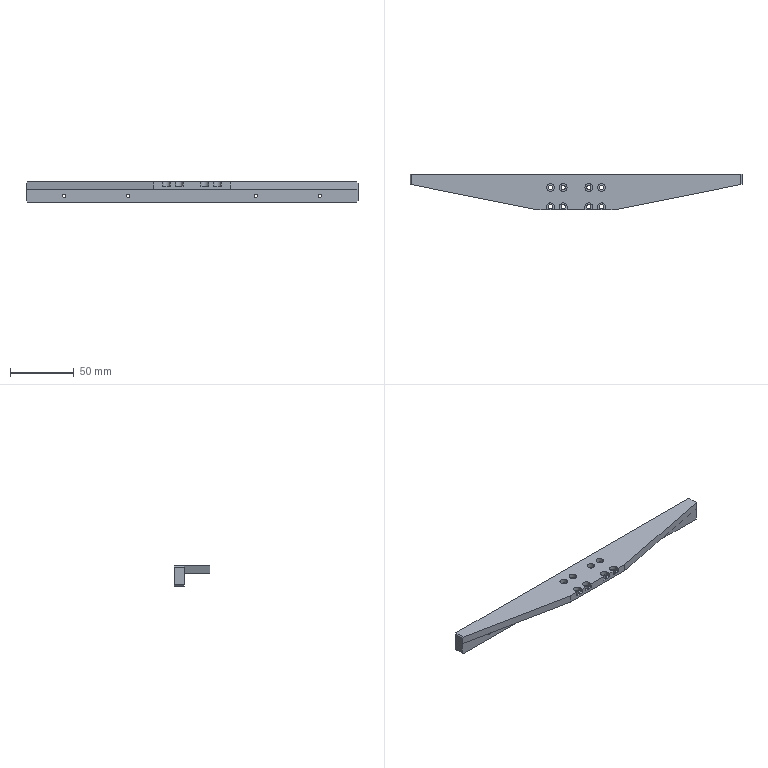NC program | NX | posted with a generic post | part box 260 x 28 x 16 mm
Whole program:
N10 G17 G21 G94 G90
(FLOOR_WALL , TOOL : D80)
N12 T19 M6
N14 G54
N16 G17 G0 G90 X-176. Y0. B0. C0. S6500 M3
N18 G43 Z30. H19
N20 Z3.
N22 G94 G1 Z0. F1500.
N24 X-173.
N26 X173.
N28 X176.
N30 Z3.
N32 G0 Z30.
N34 M5
(CAVITY_MILL , TOOL : D10)
N36 T15 M6
N38 G54
N40 G17 G0 G90 X4.33 Y-23.997 B0. C0. S9500 M3
N42 G43 Z30. H15
N44 Z0.51
N46 G94 G1 Z-0.99 F1000.
N48 X0.866 Y-17.997
N50 G3 X0. Y-17.497 R1.
N52 G1 X-132.949 F3500.
N54 X-132.995 Y-17.498
N56 G2 X-133.497 Y-16.977 R0.497
N58 G1 Y0.761
N60 G2 X-136.298 Y6. R6.301
N62 G1 Y13.727
N64 X-136.299 Y13.788
N66 Y14.001
N68 G2 X-129.99 Y20.3 R6.305
N70 G1 X129.99
N72 G2 X136.299 Y14. R6.305
N74 G1 Y6.004
N76 G2 X134.23 Y1.333 R6.307
N78 X133.497 Y0.761 R6.297
N80 G1 Y-16.999
N82 G2 X132.995 Y-17.498 R0.497
N84 G1 X132.949 Y-17.497
N86 X0.
N88 Y-11.497
N90 X-127.497
N92 Y-0.3
N94 X127.497
N96 Y0.9
N98 X-129.99
N100 G2 X-135.098 Y6. R5.101
N102 G1 Y13.774
N104 X-135.099 Y13.788
N106 Y14.
N108 G2 X-129.99 Y19.1 R5.105
N110 G1 X129.99
N112 G2 X135.099 Y14. R5.105
N114 G1 Y6.004
N116 G2 X133.424 Y2.222 R5.107
N118 X130. Y0.9 R5.097
N120 G1 X127.497
N122 Y-0.3
N124 Y-11.497
N126 X0.
N128 Y-6.997
N130 X-122.997
N132 Y-4.8
N134 X122.997
N136 Y-6.997
N138 X0.
N140 G3 X-0.866 Y-7.497 R1.
N142 G1 Z0.51
N144 G0 X4.33 Y-23.998 Z-0.48
N146 G1 Z-1.98 F1000.
N148 X0.866 Y-17.998
N150 G3 X0. Y-17.498 R1.
N152 G1 X-132.949 F3500.
N154 X-132.995
N156 G2 X-133.497 Y-16.977 R0.497
N158 G1 Y0.76
N160 G2 X-136.3 Y6. R6.3
N162 G1 Y14.
N164 G2 X-130. Y20.3 R6.3
N166 G1 X130.
N168 G2 X136.3 Y14. R6.3
N170 G1 Y6.
N172 G2 X133.497 Y0.76 R6.3
N174 G1 Y-16.999
N176 G2 X132.995 Y-17.498 R0.497
N178 G1 X132.949
N180 X0.
N182 Y-11.498
N184 X-127.497
N186 Y-0.3
N188 X127.497
N190 Y0.9
N192 X-130.
N194 G2 X-135.1 Y6. R5.1
N196 G1 Y14.
N198 G2 X-130. Y19.1 R5.1
N200 G1 X130.
N202 G2 X135.1 Y14. R5.1
N204 G1 Y6.
N206 G2 X130. Y0.9 R5.1
N208 G1 X127.497
N210 Y-0.3
N212 Y-11.498
N214 X0.
N216 Y-6.998
N218 X-122.997
N220 Y-4.8
N222 X122.997
N224 Y-6.998
N226 X0.
N228 G3 X-0.866 Y-7.498 R1.
N230 G1 Z-0.48
N232 G0 X4.33 Y-23.998 Z-1.47
N234 G1 Z-2.97 F1000.
N236 X0.866 Y-17.998
N238 G3 X0. Y-17.498 R1.
N240 G1 X-132.949 F3500.
N242 X-132.995
N244 G2 X-133.497 Y-16.977 R0.497
N246 G1 Y0.76
N248 G2 X-136.3 Y6. R6.3
N250 G1 Y14.
N252 G2 X-130. Y20.3 R6.3
N254 G1 X130.
N256 G2 X136.3 Y14. R6.3
N258 G1 Y6.
N260 G2 X133.497 Y0.76 R6.3
N262 G1 Y-16.999
N264 G2 X132.995 Y-17.498 R0.497
N266 G1 X132.949
N268 X0.
N270 Y-11.498
N272 X-127.497
N274 Y-0.3
N276 X127.497
N278 Y0.9
N280 X-130.
N282 G2 X-135.1 Y6. R5.1
N284 G1 Y14.
N286 G2 X-130. Y19.1 R5.1
N288 G1 X130.
N290 G2 X135.1 Y14. R5.1
N292 G1 Y6.
N294 G2 X130. Y0.9 R5.1
N296 G1 X127.497
N298 Y-0.3
N300 Y-11.498
N302 X0.
N304 Y-6.998
N306 X-122.997
N308 Y-4.8
N310 X122.997
N312 Y-6.998
N314 X0.
N316 G3 X-0.866 Y-7.498 R1.
N318 G1 Z-1.47
N320 G0 X4.33 Y-23.998 Z-2.46
N322 G1 Z-3.96 F1000.
N324 X0.866 Y-17.998
N326 G3 X0. Y-17.498 R1.
N328 G1 X-132.949 F3500.
N330 X-132.995
N332 G2 X-133.497 Y-16.977 R0.497
N334 G1 Y0.76
N336 G2 X-136.3 Y6. R6.3
N338 G1 Y14.
N340 G2 X-130. Y20.3 R6.3
N342 G1 X130.
N344 G2 X136.3 Y14. R6.3
N346 G1 Y6.
N348 G2 X133.498 Y0.76 R6.3
N350 G1 Y-16.998
N352 G2 X132.995 Y-17.498 R0.497
N354 G1 X132.949
N356 X0.
N358 Y-11.498
N360 X-127.497
N362 Y-0.3
N364 X127.498
N366 Y0.9
N368 X-130.
N370 G2 X-135.1 Y6. R5.1
N372 G1 Y14.
N374 G2 X-130. Y19.1 R5.1
N376 G1 X130.
N378 G2 X135.1 Y14. R5.1
N380 G1 Y6.
N382 G2 X130. Y0.9 R5.1
N384 G1 X127.498
N386 Y-0.3
N388 Y-11.498
N390 X0.
N392 Y-6.998
N394 X-122.997
N396 Y-4.8
N398 X122.998
N400 Y-6.998
N402 X0.
N404 G3 X-0.866 Y-7.498 R1.
N406 G1 Z-2.46
N408 G0 X4.33 Y-23.998 Z-3.45
N410 G1 Z-4.95 F1000.
N412 X0.866 Y-17.998
N414 G3 X0. Y-17.498 R1.
N416 G1 X-132.949 F3500.
N418 X-132.995
N420 G2 X-133.497 Y-16.977 R0.497
N422 G1 Y0.76
N424 G2 X-136.3 Y6. R6.3
N426 G1 Y14.
N428 G2 X-130. Y20.3 R6.3
N430 G1 X130.
N432 G2 X136.3 Y14. R6.3
N434 G1 Y6.
N436 G2 X133.498 Y0.76 R6.3
N438 G1 Y-16.998
N440 G2 X132.995 Y-17.498 R0.498
N442 G1 X132.949
N444 X0.
N446 Y-11.498
N448 X-127.497
N450 Y-0.3
N452 X127.498
N454 Y0.9
N456 X-130.
N458 G2 X-135.1 Y6. R5.1
N460 G1 Y14.
N462 G2 X-130. Y19.1 R5.1
N464 G1 X130.
N466 G2 X135.1 Y14. R5.1
N468 G1 Y6.
N470 G2 X130. Y0.9 R5.1
N472 G1 X127.498
N474 Y-0.3
N476 Y-11.498
N478 X0.
N480 Y-6.998
N482 X-122.997
N484 Y-4.8
N486 X122.998
N488 Y-6.998
N490 X0.
N492 G3 X-0.866 Y-7.498 R1.
N494 G1 Z-3.45
N496 G0 X4.33 Y-23.998 Z-4.44
N498 G1 Z-5.94 F1000.
N500 X0.866 Y-17.998
N502 G3 X0. Y-17.498 R1.
N504 G1 X-132.949 F3500.
N506 X-132.995
N508 G2 X-133.497 Y-16.977 R0.498
N510 G1 Y0.76
N512 G2 X-136.3 Y6. R6.3
N514 G1 Y14.
N516 G2 X-130. Y20.3 R6.3
N518 G1 X130.
N520 G2 X136.3 Y14. R6.3
N522 G1 Y6.
N524 G2 X133.498 Y0.76 R6.3
N526 G1 Y-16.998
N528 G2 X132.995 Y-17.498 R0.498
N530 G1 X132.949
N532 X0.
N534 Y-11.498
N536 X-127.497
N538 Y-0.3
N540 X127.498
N542 Y0.9
N544 X-130.
N546 G2 X-135.1 Y6. R5.1
N548 G1 Y14.
N550 G2 X-130. Y19.1 R5.1
N552 G1 X130.
N554 G2 X135.1 Y14. R5.1
N556 G1 Y6.
N558 G2 X130. Y0.9 R5.1
N560 G1 X127.498
N562 Y-0.3
N564 Y-11.498
N566 X0.
N568 Y-6.998
N570 X-122.997
N572 Y-4.8
N574 X122.998
N576 Y-6.998
N578 X0.
N580 G3 X-0.866 Y-7.498 R1.
N582 G1 Z-4.44
N584 G0 X4.331 Y-23.998 Z-5.43
N586 G1 Z-6.93 F1000.
N588 X0.866 Y-17.998
N590 G3 X0. Y-17.498 R1.
N592 G1 X-132.949 F3500.
N594 X-132.995
N596 G2 X-133.497 Y-16.977 R0.498
N598 G1 Y0.76
N600 G2 X-136.3 Y6. R6.3
N602 G1 Y14.
N604 G2 X-130. Y20.3 R6.3
N606 G1 X130.
N608 G2 X136.3 Y14. R6.3
N610 G1 Y6.
N612 G2 X133.498 Y0.76 R6.3
N614 G1 Y-16.998
N616 G2 X132.995 Y-17.498 R0.498
N618 G1 X132.949
N620 X0.
N622 Y-11.498
N624 X-127.497
N626 Y-0.3
N628 X127.498
N630 Y0.9
N632 X-130.
N634 G2 X-135.1 Y6. R5.1
N636 G1 Y14.
N638 G2 X-130. Y19.1 R5.1
N640 G1 X130.
N642 G2 X135.1 Y14. R5.1
N644 G1 Y6.
N646 G2 X130. Y0.9 R5.1
N648 G1 X127.498
N650 Y-0.3
N652 Y-11.498
N654 X0.
N656 Y-6.998
N658 X-122.997
N660 Y-4.8
N662 X122.998
N664 Y-6.998
N666 X0.
N668 G3 X-0.866 Y-7.498 R1.
N670 G1 Z-5.43
N672 G0 X4.331 Y-23.998 Z-6.42
N674 G1 Z-7.92 F1000.
N676 X0.866 Y-17.998
N678 G3 X0. Y-17.498 R1.
N680 G1 X-132.949 F3500.
N682 X-132.995
N684 G2 X-133.497 Y-16.977 R0.498
N686 G1 Y0.76
N688 G2 X-136.3 Y6. R6.3
N690 G1 Y14.
N692 G2 X-130. Y20.3 R6.3
N694 G1 X130.
N696 G2 X136.3 Y14. R6.3
N698 G1 Y6.
N700 G2 X133.498 Y0.761 R6.3
N702 G1 Y-16.998
N704 G2 X132.995 Y-17.498 R0.498
N706 G1 X132.949
N708 X0.
N710 Y-11.498
N712 X-127.497
N714 Y-0.3
N716 X127.498
N718 Y0.9
N720 X-130.
N722 G2 X-135.1 Y6. R5.1
N724 G1 Y14.
N726 G2 X-130. Y19.1 R5.1
N728 G1 X130.
N730 G2 X135.1 Y14. R5.1
N732 G1 Y6.
N734 G2 X130. Y0.9 R5.1
N736 G1 X127.498
N738 Y-0.3
N740 Y-11.498
N742 X0.
N744 Y-6.998
N746 X-122.997
N748 Y-4.8
N750 X122.998
N752 Y-6.998
N754 X0.
N756 G3 X-0.866 Y-7.498 R1.
N758 G1 Z-6.42
N760 G0 X4.331 Y-23.998 Z-7.41
N762 G1 Z-8.91 F1000.
N764 X0.867 Y-17.998
N766 G3 X0.001 Y-17.498 R1.
N768 G1 X-132.949 F3500.
N770 X-132.995
N772 G2 X-133.498 Y-16.977 R0.498
N774 G1 Y0.76
N776 G2 X-136.3 Y6. R6.3
N778 G1 Y14.
N780 G2 X-130. Y20.3 R6.3
N782 G1 X130.
N784 G2 X136.3 Y14. R6.3
N786 G1 Y6.
N788 G2 X133.499 Y0.761 R6.3
N790 G1 Y-16.998
N792 G2 X132.995 Y-17.498 R0.499
N794 G1 X132.949
N796 X0.001
N798 Y-11.498
N800 X-127.498
N802 Y-0.3
N804 X127.499
N806 Y0.9
N808 X-130.
N810 G2 X-135.1 Y6. R5.1
N812 G1 Y14.
N814 G2 X-130. Y19.1 R5.1
N816 G1 X130.
N818 G2 X135.1 Y14. R5.1
N820 G1 Y6.
N822 G2 X130. Y0.9 R5.1
N824 G1 X127.499
N826 Y-0.3
N828 Y-11.498
N830 X0.001
N832 Y-6.998
N834 X-122.998
N836 Y-4.8
N838 X122.999
N840 Y-6.998
N842 X0.001
N844 G3 X-0.866 Y-7.498 R1.
N846 G1 Z-7.41
N848 G0 X4.331 Y-23.998 Z-8.4
N850 G1 Z-9.9 F1000.
N852 X0.867 Y-17.998
N854 G3 X0.001 Y-17.498 R1.
N856 G1 X-132.949 F3500.
N858 X-132.995 Y-17.499
N860 G2 X-133.498 Y-16.977 R0.498
N862 G1 Y0.76
N864 G2 X-136.3 Y6. R6.3
N866 G1 Y14.
N868 G2 X-130. Y20.3 R6.3
N870 G1 X130.
N872 G2 X136.3 Y14. R6.3
N874 G1 Y6.
N876 G2 X133.499 Y0.761 R6.3
N878 G1 Y-16.998
N880 G2 X132.995 Y-17.499 R0.499
N882 G1 X132.949 Y-17.498
N884 X0.001
N886 Y-11.498
N888 X-127.498
N890 Y-0.3
N892 X127.499
N894 Y0.9
N896 X-130.
N898 G2 X-135.1 Y6. R5.1
N900 G1 Y14.
N902 G2 X-130. Y19.1 R5.1
N904 G1 X130.
N906 G2 X135.1 Y14. R5.1
N908 G1 Y6.
N910 G2 X130. Y0.9 R5.1
N912 G1 X127.499
N914 Y-0.3
N916 Y-11.498
N918 X0.001
N920 Y-6.998
N922 X-122.998
N924 Y-4.8
N926 X122.999
N928 Y-6.998
N930 X0.001
N932 G3 X-0.865 Y-7.498 R1.
N934 G1 Z-8.4
N936 G0 X125.868 Y-23.998 Z-9.271
N938 G1 Z-10.771 F1000.
N940 X122.404 Y-17.998
N942 G3 X121.538 Y-17.498 R1.
N944 G1 X44.632 F3500.
N946 X31.236 Y-20.178
N948 G2 X30. Y-20.3 R6.3
N950 G1 X-30.
N952 G2 X-31.236 Y-20.178 R6.3
N954 G1 X-44.632 Y-17.498
N956 X-132.949
N958 X-132.995 Y-17.499
N960 G2 X-133.498 Y-16.977 R0.498
N962 G1 Y-0.925
N964 X-127.498
N966 X-74.632 Y-11.498
N968 X-127.498
N970 Y-0.925
N972 X-122.998 Y-6.414
N974 X-120.077 Y-6.998
N976 X-122.998
N978 Y-6.414
N980 X-127.498 Y-0.925
N982 X-133.498
N984 Y0.76
N986 G2 X-136.3 Y6. R6.3
N988 G1 Y14.
N990 G2 X-130. Y20.3 R6.3
N992 G1 X130.
N994 G2 X136.3 Y14. R6.3
N996 G1 Y6.
N998 G2 X133.499 Y0.761 R6.3
N1000 G1 Y-16.997
N1002 G2 X132.995 Y-17.499 R0.499
N1004 G1 X132.949 Y-17.498
N1006 X121.538
N1008 Y-11.498
N1010 X74.632
N1012 X127.499 Y-0.925
N1014 X127.264 Y0.252
N1016 X31. Y-19.001
N1018 G2 X30. Y-19.1 R5.1
N1020 G1 X-30.
N1022 G2 X-31. Y-19.001 R5.1
N1024 G1 X-131. Y0.999
N1026 G2 X-135.1 Y6. R5.1
N1028 G1 Y14.
N1030 G2 X-130. Y19.1 R5.1
N1032 G1 X130.
N1034 G2 X135.1 Y14. R5.1
N1036 G1 Y6.
N1038 G2 X131. Y0.999 R5.1
N1040 G1 X127.264 Y0.252
N1042 X127.499 Y-0.925
N1044 Y-11.498
N1046 X121.538
N1048 Y-6.998
N1050 X120.077
N1052 X122.999 Y-6.414
N1054 Y-6.998
N1056 X121.538
N1058 G3 X120.672 Y-7.498 R1.
N1060 G1 Z-9.271
N1062 G0 X125.868 Y-23.999 Z-10.143
N1064 G1 Z-11.643 F1000.
N1066 X122.404 Y-17.999
N1068 G3 X121.538 Y-17.499 R1.
N1070 G1 X44.631 F3500.
N1072 X31.236 Y-20.178
N1074 G2 X30. Y-20.3 R6.3
N1076 G1 X-30.
N1078 G2 X-31.236 Y-20.178 R6.3
N1080 G1 X-44.631 Y-17.499
N1082 X-132.949
N1084 X-132.995
N1086 G2 X-133.498 Y-16.977 R0.499
N1088 G1 Y-0.925
N1090 X-127.498
N1092 X-74.631 Y-11.499
N1094 X-127.498
N1096 Y-0.925
N1098 X-122.998 Y-6.414
N1100 X-120.077 Y-6.999
N1102 X-122.998
N1104 Y-6.414
N1106 X-127.498 Y-0.925
N1108 X-133.498
N1110 Y0.76
N1112 G2 X-136.3 Y6. R6.3
N1114 G1 Y14.
N1116 G2 X-130. Y20.3 R6.3
N1118 G1 X130.
N1120 G2 X136.3 Y14. R6.3
N1122 G1 Y6.
N1124 G2 X133.499 Y0.761 R6.3
N1126 G1 Y-16.997
N1128 G2 X132.995 Y-17.499 R0.499
N1130 G1 X132.949
N1132 X121.538
N1134 Y-11.499
N1136 X74.631
N1138 X127.499 Y-0.925
N1140 X127.264 Y0.252
N1142 X31. Y-19.001
N1144 G2 X30. Y-19.1 R5.1
N1146 G1 X-30.
N1148 G2 X-31. Y-19.001 R5.1
N1150 G1 X-131. Y0.999
N1152 G2 X-135.1 Y6. R5.1
N1154 G1 Y14.
N1156 G2 X-130. Y19.1 R5.1
N1158 G1 X130.
N1160 G2 X135.1 Y14. R5.1
N1162 G1 Y6.
N1164 G2 X131. Y0.999 R5.1
N1166 G1 X127.264 Y0.252
N1168 X127.499 Y-0.925
N1170 Y-11.499
N1172 X121.538
N1174 Y-6.999
N1176 X120.077
N1178 X122.999 Y-6.414
N1180 Y-6.999
N1182 X121.538
N1184 G3 X120.672 Y-7.499 R1.
N1186 G1 Z-10.143
N1188 G0 X125.868 Y-23.999 Z-11.014
N1190 G1 Z-12.514 F1000.
N1192 X122.404 Y-17.999
N1194 G3 X121.538 Y-17.499 R1.
N1196 G1 X44.631 F3500.
N1198 X31.236 Y-20.178
N1200 G2 X30. Y-20.3 R6.3
N1202 G1 X-30.
N1204 G2 X-31.236 Y-20.178 R6.3
N1206 G1 X-44.631 Y-17.499
N1208 X-132.949
N1210 X-132.995
N1212 G2 X-133.498 Y-16.977 R0.499
N1214 G1 Y-0.925
N1216 X-127.498
N1218 X-74.631 Y-11.499
N1220 X-127.498
N1222 Y-0.925
N1224 X-122.998 Y-6.414
N1226 X-120.076 Y-6.999
N1228 X-122.998
N1230 Y-6.414
N1232 X-127.498 Y-0.925
N1234 X-133.498
N1236 Y0.76
N1238 G2 X-136.3 Y6. R6.3
N1240 G1 Y14.
N1242 G2 X-130. Y20.3 R6.3
N1244 G1 X130.
N1246 G2 X136.3 Y14. R6.3
N1248 G1 Y6.
N1250 G2 X133.499 Y0.761 R6.3
N1252 G1 Y-16.997
N1254 G2 X132.995 Y-17.499 R0.499
N1256 G1 X132.949
N1258 X121.538
N1260 Y-11.499
N1262 X74.631
N1264 X127.499 Y-0.925
N1266 X127.264 Y0.252
N1268 X31. Y-19.001
N1270 G2 X30. Y-19.1 R5.1
N1272 G1 X-30.
N1274 G2 X-31. Y-19.001 R5.1
N1276 G1 X-131. Y0.999
N1278 G2 X-135.1 Y6. R5.1
N1280 G1 Y14.
N1282 G2 X-130. Y19.1 R5.1
N1284 G1 X130.
N1286 G2 X135.1 Y14. R5.1
N1288 G1 Y6.
N1290 G2 X131. Y0.999 R5.1
N1292 G1 X127.264 Y0.252
N1294 X127.499 Y-0.925
N1296 Y-11.499
N1298 X121.538
N1300 Y-6.999
N1302 X120.076
N1304 X122.999 Y-6.414
N1306 Y-6.999
N1308 X121.538
N1310 G3 X120.672 Y-7.499 R1.
N1312 G1 Z-11.014
N1314 G0 X125.868 Y-23.999 Z-11.886
N1316 G1 Z-13.386 F1000.
N1318 X122.404 Y-17.999
N1320 G3 X121.538 Y-17.499 R1.
N1322 G1 X44.63 F3500.
N1324 X31.236 Y-20.178
N1326 G2 X30. Y-20.3 R6.3
N1328 G1 X-30.
N1330 G2 X-31.236 Y-20.178 R6.3
N1332 G1 X-44.63 Y-17.499
N1334 X-132.949
N1336 X-132.995
N1338 G2 X-133.498 Y-16.977 R0.499
N1340 G1 Y-0.925
N1342 X-127.498
N1344 X-74.63 Y-11.499
N1346 X-127.498
N1348 Y-0.925
N1350 X-122.998 Y-6.414
N1352 X-120.076 Y-6.999
N1354 X-122.998
N1356 Y-6.414
N1358 X-127.498 Y-0.925
N1360 X-133.498
N1362 Y0.76
N1364 G2 X-136.3 Y6. R6.3
N1366 G1 Y14.
N1368 G2 X-130. Y20.3 R6.3
N1370 G1 X130.
N1372 G2 X136.3 Y14. R6.3
N1374 G1 Y6.
N1376 G2 X133.499 Y0.761 R6.3
N1378 G1 X133.5 Y-16.997
N1380 G2 X132.995 Y-17.499 R0.5
N1382 G1 X132.949
N1384 X121.538
N1386 Y-11.499
N1388 X74.63
N1390 X127.499 Y-0.925
N1392 X127.264 Y0.252
N1394 X31. Y-19.001
N1396 G2 X30. Y-19.1 R5.1
N1398 G1 X-30.
N1400 G2 X-31. Y-19.001 R5.1
N1402 G1 X-131. Y0.999
N1404 G2 X-135.1 Y6. R5.1
N1406 G1 Y14.
N1408 G2 X-130. Y19.1 R5.1
N1410 G1 X130.
N1412 G2 X135.1 Y14. R5.1
N1414 G1 Y6.
N1416 G2 X131. Y0.999 R5.1
N1418 G1 X127.264 Y0.252
N1420 X127.499 Y-0.925
N1422 Y-11.499
N1424 X121.538
N1426 Y-6.999
N1428 X120.076
N1430 X122.999 Y-6.414
N1432 Y-6.999
N1434 X121.538
N1436 G3 X120.672 Y-7.499 R1.
N1438 G1 Z-11.886
N1440 G0 X125.868 Y-23.999 Z-12.757
N1442 G1 Z-14.257 F1000.
N1444 X122.404 Y-17.999
N1446 G3 X121.538 Y-17.499 R1.
N1448 G1 X44.63 F3500.
N1450 X31.236 Y-20.178
N1452 G2 X30. Y-20.3 R6.3
N1454 G1 X-30.
N1456 G2 X-31.236 Y-20.178 R6.3
N1458 G1 X-44.63 Y-17.499
N1460 X-132.949
N1462 X-132.995
N1464 G2 X-133.498 Y-16.977 R0.499
N1466 G1 Y-0.925
N1468 X-127.498
N1470 X-74.63 Y-11.499
N1472 X-127.498
N1474 Y-0.925
N1476 X-122.998 Y-6.414
N1478 X-120.076 Y-6.999
N1480 X-122.998
N1482 Y-6.414
N1484 X-127.498 Y-0.925
N1486 X-133.498
N1488 Y0.76
N1490 G2 X-136.3 Y6. R6.3
N1492 G1 Y14.
N1494 G2 X-130. Y20.3 R6.3
N1496 G1 X130.
N1498 G2 X136.3 Y14. R6.3
N1500 G1 Y6.
N1502 G2 X133.5 Y0.761 R6.3
N1504 G1 Y-16.997
N1506 G2 X132.995 Y-17.499 R0.5
N1508 G1 X132.949
N1510 X121.538
N1512 Y-11.499
N1514 X74.63
N1516 X127.5 Y-0.925
N1518 X127.264 Y0.252
N1520 X31. Y-19.001
N1522 G2 X30. Y-19.1 R5.1
N1524 G1 X-30.
N1526 G2 X-31. Y-19.001 R5.1
N1528 G1 X-131. Y0.999
N1530 G2 X-135.1 Y6. R5.1
N1532 G1 Y14.
N1534 G2 X-130. Y19.1 R5.1
N1536 G1 X130.
N1538 G2 X135.1 Y14. R5.1
N1540 G1 Y6.
N1542 G2 X131. Y0.999 R5.1
N1544 G1 X127.264 Y0.252
N1546 X127.5 Y-0.925
N1548 Y-11.499
N1550 X121.538
N1552 Y-6.999
N1554 X120.076
N1556 X123. Y-6.414
N1558 Y-6.999
N1560 X121.538
N1562 G3 X120.672 Y-7.499 R1.
N1564 G1 Z-12.757
N1566 G0 X125.868 Y-23.999 Z-13.629
N1568 G1 Z-15.129 F1000.
N1570 X122.403 Y-17.999
N1572 G3 X121.537 Y-17.499 R1.
N1574 G1 X44.629 F3500.
N1576 X31.236 Y-20.178
N1578 G2 X30. Y-20.3 R6.3
N1580 G1 X-30.
N1582 G2 X-31.236 Y-20.178 R6.3
N1584 G1 X-44.629 Y-17.499
N1586 X-132.949
N1588 X-132.995
N1590 G2 X-133.498 Y-16.977 R0.499
N1592 G1 Y-0.925
N1594 X-127.498
N1596 X-74.629 Y-11.499
N1598 X-127.498
N1600 Y-0.925
N1602 X-122.998 Y-6.414
N1604 X-120.075 Y-6.999
N1606 X-122.998
N1608 Y-6.414
N1610 X-127.498 Y-0.925
N1612 X-133.498
N1614 Y0.76
N1616 G2 X-136.3 Y6. R6.3
N1618 G1 Y14.
N1620 G2 X-130. Y20.3 R6.3
N1622 G1 X130.
N1624 G2 X136.3 Y14. R6.3
N1626 G1 Y6.
N1628 G2 X133.5 Y0.762 R6.3
N1630 G1 Y-16.997
N1632 G2 X132.995 Y-17.499 R0.5
N1634 G1 X132.949
N1636 X121.537
N1638 Y-11.499
N1640 X74.629
N1642 X127.5 Y-0.925
N1644 X127.264 Y0.252
N1646 X31. Y-19.001
N1648 G2 X30. Y-19.1 R5.1
N1650 G1 X-30.
N1652 G2 X-31. Y-19.001 R5.1
N1654 G1 X-131. Y0.999
N1656 G2 X-135.1 Y6. R5.1
N1658 G1 Y14.
N1660 G2 X-130. Y19.1 R5.1
N1662 G1 X130.
N1664 G2 X135.1 Y14. R5.1
N1666 G1 Y6.
N1668 G2 X131. Y0.999 R5.1
N1670 G1 X127.264 Y0.252
N1672 X127.5 Y-0.925
N1674 Y-11.499
N1676 X121.537
N1678 Y-6.999
N1680 X120.075
N1682 X123. Y-6.414
N1684 Y-6.999
N1686 X121.537
N1688 G3 X120.671 Y-7.499 R1.
N1690 G1 Z-13.629
N1692 G0 X125.867 Y-23.999 Z-14.5
N1694 G1 Z-16. F1000.
N1696 X122.403 Y-17.999
N1698 G3 X121.537 Y-17.499 R1.
N1700 G1 X44.629 F3500.
N1702 X31.236 Y-20.178
N1704 G2 X30. Y-20.3 R6.3
N1706 G1 X-30.
N1708 G2 X-31.236 Y-20.178 R6.3
N1710 G1 X-44.629 Y-17.499
N1712 X-132.949
N1714 X-132.995
N1716 G2 X-133.498 Y-16.977 R0.499
N1718 G1 Y-0.925
N1720 X-127.498
N1722 X-74.629 Y-11.499
N1724 X-127.498
N1726 Y-0.925
N1728 X-122.998 Y-6.414
N1730 X-120.075 Y-6.999
N1732 X-122.998
N1734 Y-6.414
N1736 X-127.498 Y-0.925
N1738 X-133.498
N1740 Y0.761
N1742 G2 X-136.3 Y6. R6.3
N1744 G1 Y14.
N1746 G2 X-130. Y20.3 R6.3
N1748 G1 X130.
N1750 G2 X136.3 Y14. R6.3
N1752 G1 Y6.
N1754 G2 X133.5 Y0.762 R6.3
N1756 G1 Y-16.997
N1758 G2 X132.995 Y-17.499 R0.5
N1760 G1 X132.949
N1762 X121.537
N1764 Y-11.499
N1766 X74.629
N1768 X127.5 Y-0.925
N1770 X127.265 Y0.252
N1772 X31. Y-19.001
N1774 G2 X30. Y-19.1 R5.1
N1776 G1 X-30.
N1778 G2 X-31. Y-19.001 R5.1
N1780 G1 X-131. Y0.999
N1782 G2 X-135.1 Y6. R5.1
N1784 G1 Y14.
N1786 G2 X-130. Y19.1 R5.1
N1788 G1 X130.
N1790 G2 X135.1 Y14. R5.1
N1792 G1 Y6.
N1794 G2 X131. Y0.999 R5.1
N1796 G1 X127.265 Y0.252
N1798 X127.5 Y-0.925
N1800 Y-11.499
N1802 X121.537
N1804 Y-6.999
N1806 X120.075
N1808 X123. Y-6.414
N1810 Y-6.999
N1812 X121.537
N1814 G3 X120.671 Y-7.499 R1.
N1816 G1 Z-14.5
N1818 G0 Z30.
N1820 M5
(ZLEVEL_PROFILE , TOOL : D10JING)
N1822 T14 M6
N1824 G54
N1826 G17 G0 G90 X132.926 Y-0.359 B0. C0. S9500 M3
N1828 G43 Z30. H14
N1830 Z-14.5
N1832 G94 G1 Z-16. F1000.
N1834 X131.928 Y0.777
N1836 G3 X130.981 Y1.097 R1.
N1838 G1 X30.981 Y-18.903 F1500.
N1840 G2 X30. Y-19. R5.
N1842 G1 X-30.
N1844 G2 X-30.981 Y-18.903 R5.
N1846 G1 X-130.981 Y1.097
N1848 G2 X-135. Y6. R5.
N1850 G1 Y14.
N1852 G2 X-130. Y19. R5.
N1854 G1 X130.
N1856 G2 X135. Y14. R5.
N1858 G1 Y6.
N1860 G2 X130.981 Y1.097 R5.
N1862 G3 X130.229 Y0.437 R1.
N1864 G1 X129.674 Y-1.204
N1866 Z-14.5
N1868 G0 Z30.
(FLOOR_WALL_1 , TOOL : D10JING)
N1870 X31.805 Y-20.268
N1872 Z-8.5
N1874 G1 Z-10. F1250.
N1876 X31.361 Y-19.5
N1878 G3 X30.495 Y-19. R1.
N1880 G1 X-30.495
N1882 X-54.87 Y-14.125
N1884 X54.87
N1886 X79.245 Y-9.25
N1888 X-79.245
N1890 X-103.62 Y-4.375
N1892 X103.62
N1894 X127.995 Y0.5
N1896 X-127.995
N1898 G3 X-128.861 Y0. R1.
N1900 G1 X-129.304 Y-0.768
N1902 Z-8.5
N1904 G0 Z30.
N1906 X131.786 Y-0.5
N1908 Z-8.5
N1910 G1 Z-10.
N1912 X131.208 Y0.5
N1914 G3 X130.342 Y1. R1.
N1916 G1 X-130.342
N1918 G3 X-131.208 Y0.5 R1.
N1920 G1 X-131.786 Y-0.5
N1922 Z-8.5
N1924 G0 Z30.
N1926 M5
(PLANAR_MILL , TOOL : D6A45)
N1928 T01 M6
N1930 G54
N1932 G17 G0 G90 X1.27 Y3.9 B0. C0. S9500 M3
N1934 G43 Z30. H1
N1936 Z0.5
N1938 G94 G1 Z-1. F1250.
N1940 X0.866 Y4.6
N1942 G3 X0. Y5.1 R1.
N1944 G1 X-129.9
N1946 G2 X-130.9 Y6.1 R1.
N1948 G1 Y13.9
N1950 G2 X-129.9 Y14.9 R1.
N1952 G1 X129.9
N1954 G2 X130.9 Y13.9 R1.
N1956 G1 Y6.1
N1958 G2 X129.9 Y5.1 R1.
N1960 G1 X0.
N1962 G3 X-0.866 Y4.6 R1.
N1964 G1 X-1.27 Y3.9
N1966 Z0.5
N1968 G0 Z30.
(PLANAR_MILL_COPY , TOOL : D6A45)
N1970 X118.477 Y1.3
N1972 Z-9.5
N1974 G1 Z-11.
N1976 X117.563 Y2.34
N1978 G3 X117.089 Y2.5 R0.5
N1980 G1 X30.186 Y-14.881
N1982 X29.99 Y-14.9
N1984 X-29.99
N1986 X-30.186 Y-14.881
N1988 X-117.089 Y2.5
N1990 G3 X-117.563 Y2.34 R0.5
N1992 G1 X-118.477 Y1.3
N1994 Z-9.5
N1996 G0 Z30.
N1998 M5
N2000 M2